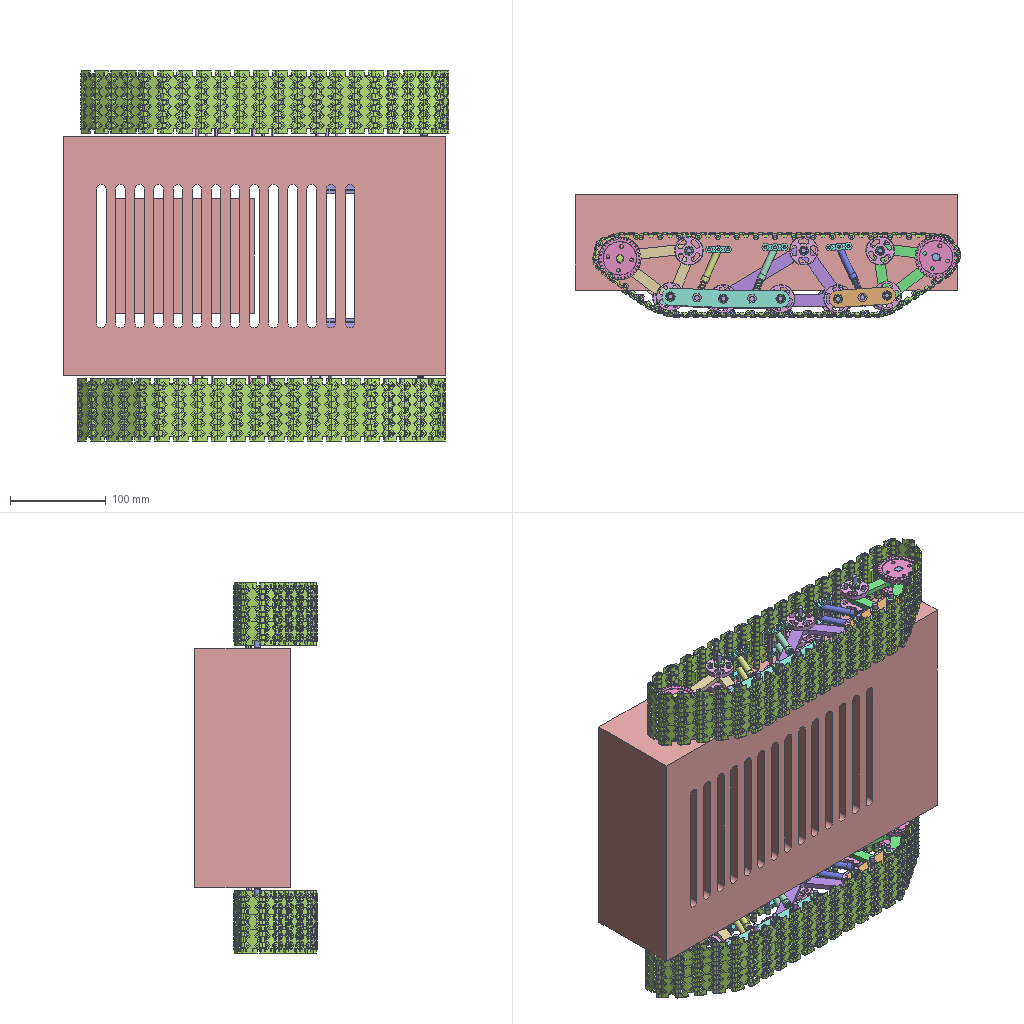Assembly | SolidWorks | 37 different items | 381 placed | box 403 x 128 x 388 mm
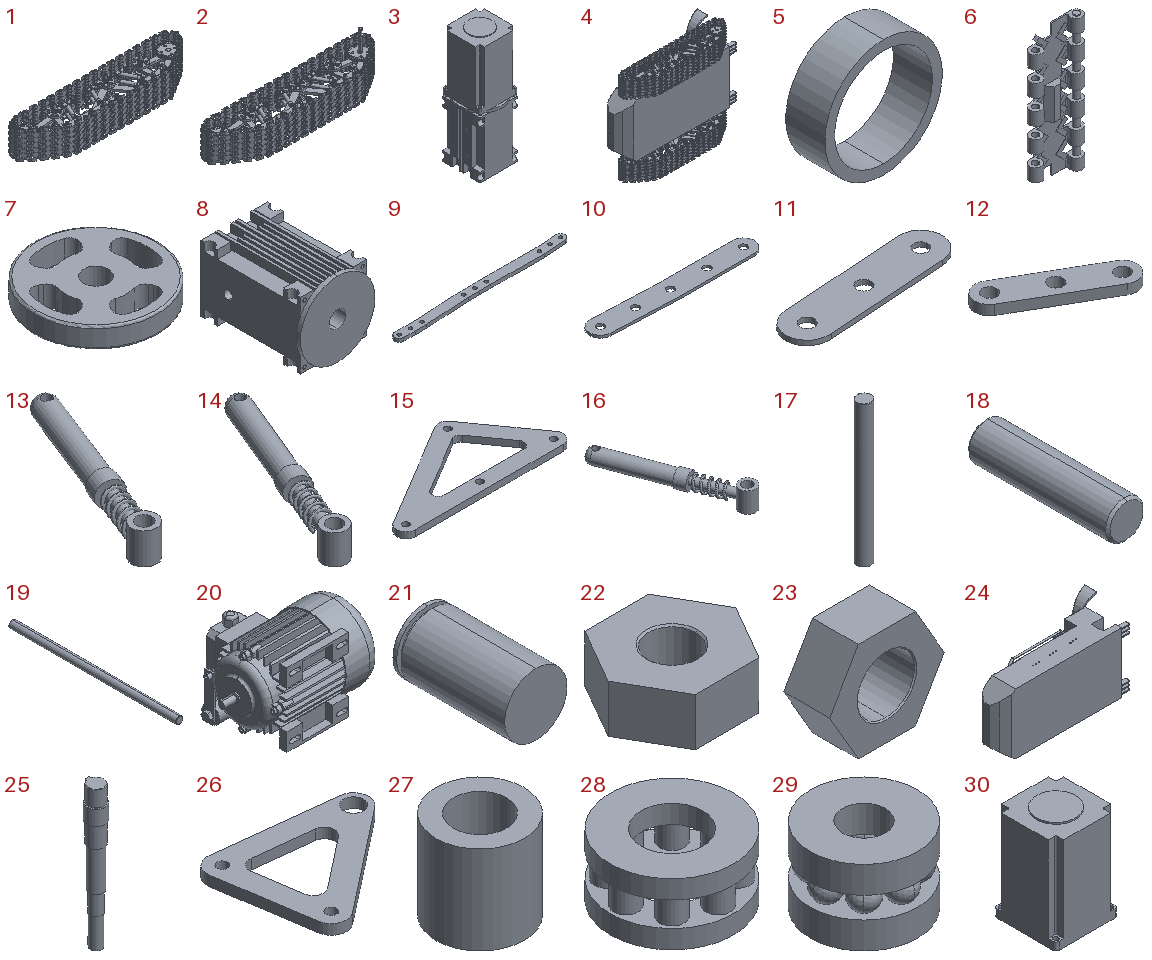Parts list (item | name | quantity | parent item | size | volume | features):
1 | (subassembly) | x1 | - | - | 270065 mm3 | features CompositeCurve 233, ReferencePattern 40, LocalChainPattern 1
2 | (subassembly) | x1 | - | - | 270065 mm3 | features CompositeCurve 245, ReferencePattern 40, LocalChainPattern 1
3 | (subassembly) | x1 | - | 45 x 45 x 123.5 mm | 175871 mm3 | -
4 | (subassembly) | x1 | - | - | 5126066 mm3 | features CompositeCurve 161, Cut 2
5 | - | x12 | in 1, 2 | 6 x 2 x 6 mm | 17.279 mm3 | features Extrusion 1
6 | - | x82 | in 1, 2 | 25.8 x 6.8 x 66 mm | 3099 mm3 | features ICE 7, Chamfer 1, Extrusion 1
7 | - | x32 | in 1, 2 | 30 x 30 x 5 mm | 2405 mm3 | features Extrusion 1, Fillet 1, ICE 1
8 | - | x1 | - | 45 x 62.5 x 45 mm | 83814 mm3 | features ICE 8, MirrorPattern 3, Extrusion 1
9 | - | x1 | - | 153.919 x 11.375 x 3 mm | 3465 mm3 | features Extrusion 1
10 | - | x4 | in 1, 2 | 133.234 x 20.271 x 2 mm | 4375 mm3 | features Extrusion 1
11 | - | x4 | in 1, 2 | 69.294 x 21.478 x 2 mm | 2186 mm3 | features Extrusion 1
12 | - | x12 | in 1, 2 | 23.321 x 16 x 2 mm | 254.137 mm3 | features Extrusion 1
13 | - | x4 | in 1, 2 | 28.061 x 59.393 x 10 mm | 2085 mm3 | features ICE 4, 3DProfileFeature 1, Extrusion 1, Fillet 1, Helix 1, Sweep 1
14 | - | x4 | in 1, 2 | 30.391 x 62.421 x 10 mm | 2131 mm3 | features ICE 4, 3DProfileFeature 2, Extrusion 1, Fillet 1, Helix 1, Sweep 1
15 | - | x2 | in 1, 2 | 135 x 65.308 x 5 mm | 17553 mm3 | features Extrusion 1
16 | - | x4 | in 1, 2 | 27.99 x 62.362 x 10 mm | 2119 mm3 | features ICE 4, 3DProfileFeature 2, Extrusion 1, Fillet 1, Helix 1, Sweep 1
17 | - | x22 | in 1, 2 | 5 x 5 x 50 mm | 981.593 mm3 | features Chamfer 1, Extrusion 1
18 | - | x2 | in 1, 2 | 8 x 30 x 8 mm | 1502 mm3 | features Chamfer 1, Extrusion 1
19 | - | x18 | - | 3 x 70 x 3 mm | 494.644 mm3 | features Extrusion 1, Fillet 1
20 | - | x1 | - | 53.612 x 38.693 x 34.5 mm | 25264 mm3 | features ICE 20, Fillet 3, CirPattern 2, Revolution 2, LPattern 1, Scale 1
21 | - | x1 | - | 150 x 290 x 150 mm | 4766313 mm3 | features ICE 3, Chamfer 1, Extrusion 1, Fillet 1
22 | - | x54 | - | 8 x 6.928 x 3 mm | 103.406 mm3 | features Chamfer 1, Extrusion 1
23 | - | x12 | in 1, 2 | 10 x 4 x 8.66 mm | 181.109 mm3 | features Chamfer 1, Extrusion 1
24 | - | x1 | - | 438.814 x 160 x 247.251 mm | 4513172 mm3 | features ICE 37, Fillet 7, Chamfer 2, 3DProfileFeature 1, BossThin 1, Extrusion 1, MirrorPattern 1, Shell 1, WeldMemberFeat 1, WeldmentFeature 1
25 | - | x2 | in 1, 2 | 9 x 9 x 71 mm | 2813 mm3 | features ICE 9, Chamfer 2, Fillet 2, Extrusion 1
26 | - | x2 | in 1, 2 | 73.414 x 61.829 x 5 mm | 9310 mm3 | features Extrusion 1
27 | - | x2 | - | 9.99 x 9.99 x 10 mm | 501.085 mm3 | features Extrusion 1
28 | - | x32 | in 1, 2 | 10 x 10 x 5 mm | 226.98 mm3 | features ICE 2, Extrusion 1
29 | - | x1 | - | 20 x 20 x 14 mm | 3133 mm3 | features CirPattern 1, Extrusion 1, ICE 1, Revolution 1
30 | - | x2 | - | 40 x 40 x 76 mm | 92058 mm3 | features ICE 4, Fillet 2, Extrusion 1
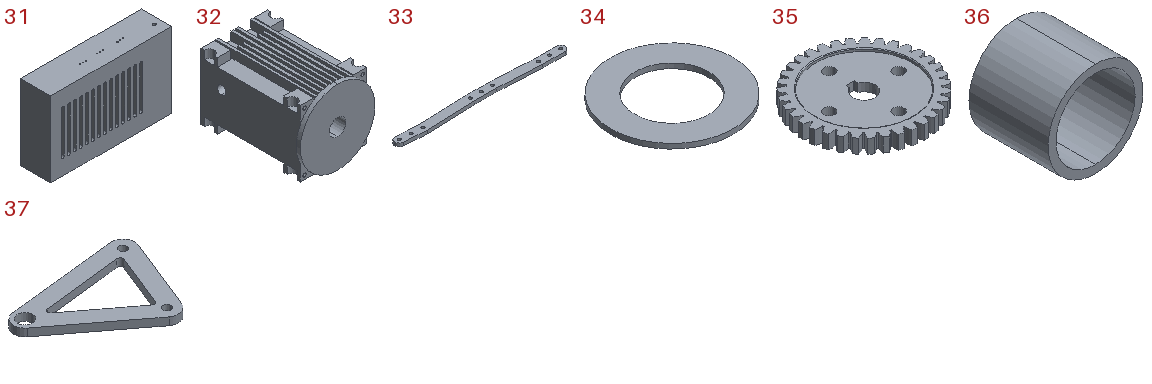31 | - | x1 | - | 400 x 100 x 250 mm | 2452161 mm3 | features ICE 7, Extrusion 1, Shell 1
32 | - | x1 | - | 45 x 62.5 x 45 mm | 83715 mm3 | features ICE 8, MirrorPattern 3, Extrusion 1
33 | - | x1 | - | 151.18 x 10.194 x 3 mm | 3447 mm3 | features Extrusion 1
34 | - | x18 | - | 5 x 5 x 0.2 mm | 2.513 mm3 | features Extrusion 1
35 | - | x8 | in 1, 2 | 44.212 x 44.202 x 5 mm | 4910 mm3 | features ICE 4, Fillet 2, Extrusion 1
36 | - | x32 | in 1, 2 | 6 x 5 x 6 mm | 43.197 mm3 | features Extrusion 1
37 | - | x2 | in 1, 2 | 87.181 x 63.036 x 5 mm | 10086 mm3 | features Extrusion 1
Mates (type | each side: item.copy, entity, surface, feature):
In the top assembly
Parallel | 31.1 edge | 10.1 edge
Concentric | 31.1 edge | 12.1 edge
Parallel | 31.1 edge | 15.1 edge
Concentric | 12.2 face cylinder Boss-Extrude1 | 19.1 edge
DistanceDim | 19.1 face plane Boss-Extrude1 | 12.2 face plane Boss-Extrude1
Concentric | 12.2 edge | 19.2 edge
DistanceDim | 19.2 face plane Boss-Extrude1 | 12.2 face plane Boss-Extrude1
Concentric | 12.2 edge | 19.3 edge
DistanceDim | 19.3 face plane Boss-Extrude1 | 12.2 face plane Boss-Extrude1
Concentric | 12.3 edge | 19.4 edge
DistanceDim | 19.4 face plane Boss-Extrude1 | 12.3 face plane Boss-Extrude1
Concentric | 12.3 edge | 19.5 edge
DistanceDim | 19.5 face plane Boss-Extrude1 | 12.3 face plane Boss-Extrude1
Concentric | 12.3 edge | 19.6 edge
DistanceDim | 19.6 face plane Boss-Extrude1 | 12.3 face plane Boss-Extrude1
Concentric | 12.4 edge | 19.7 edge
DistanceDim | 19.7 face plane Boss-Extrude1 | 12.4 face plane Boss-Extrude1
Concentric | 12.4 edge | 19.8 edge
DistanceDim | 19.8 face plane Boss-Extrude1 | 12.4 face plane Boss-Extrude1
Concentric | 12.4 edge | 19.9 edge
DistanceDim | 19.9 face plane Boss-Extrude1 | 12.4 face plane Boss-Extrude1
Concentric | 12.5 edge | 19.10 edge
DistanceDim | 19.10 face plane Boss-Extrude1 | 12.5 face plane Boss-Extrude1
DistanceDim | 19.9 face plane Boss-Extrude1 | 31.1 face plane
DistanceDim | 19.10 face plane Boss-Extrude1 | 31.1 face plane
Concentric | 12.5 edge | 19.11 edge
DistanceDim | 19.11 face plane Boss-Extrude1 | 12.5 face plane Boss-Extrude1
Concentric | 12.5 edge | 19.12 edge
DistanceDim | 19.12 face plane Boss-Extrude1 | 12.5 face plane Boss-Extrude1
Concentric | 12.6 edge | 19.13 edge
DistanceDim | 19.13 face plane Boss-Extrude1 | 12.6 face plane Boss-Extrude1
Concentric | 12.6 edge | 19.14 edge
DistanceDim | 19.14 face plane Boss-Extrude1 | 12.6 face plane Boss-Extrude1
Concentric | 12.6 edge | 19.15 edge
DistanceDim | 19.15 face plane Boss-Extrude1 | 12.6 face plane Boss-Extrude1
Concentric | 12.1 edge | 19.16 edge
DistanceDim | 19.16 face plane Boss-Extrude1 | 12.1 face plane Boss-Extrude1
Concentric | 12.1 edge | 19.17 edge
DistanceDim | 19.17 face plane Boss-Extrude1 | 12.1 face plane Boss-Extrude1
Concentric | 12.1 edge | 19.18 edge
DistanceDim | 19.18 face plane Boss-Extrude1 | 12.1 face plane Boss-Extrude1
Coincident | 12.2 face plane Boss-Extrude1 | 22.1 face plane Boss-Extrude1
Concentric | 12.2 edge | 22.1 edge
Coincident | 12.2 face plane Boss-Extrude1 | 22.2 face plane Boss-Extrude1
Concentric | 12.2 edge | 22.2 edge
Coincident | 12.2 face plane Boss-Extrude1 | 22.3 face plane Boss-Extrude1
Concentric | 12.2 edge | 22.3 edge
Coincident | 12.3 face plane Boss-Extrude1 | 22.4 face plane Boss-Extrude1
Concentric | 12.3 edge | 22.4 edge
Coincident | 12.3 face plane Boss-Extrude1 | 22.5 face plane Boss-Extrude1
Concentric | 12.3 edge | 22.5 edge
Coincident | 12.3 face plane Boss-Extrude1 | 22.6 face plane Boss-Extrude1
Concentric | 19.6 edge | 22.6 edge
Coincident | 12.4 face plane Boss-Extrude1 | 22.7 face plane Boss-Extrude1
Concentric | 12.4 edge | 22.7 edge
Coincident | 12.4 face plane Boss-Extrude1 | 22.8 face plane Boss-Extrude1
Concentric | 19.8 face cylinder Boss-Extrude1 | 22.8 edge
Coincident | 12.4 face plane Boss-Extrude1 | 22.9 face plane Boss-Extrude1
Concentric | 12.4 edge | 22.9 edge
Coincident | 12.7 face plane Boss-Extrude1 | 22.10 face plane Boss-Extrude1
Concentric | 19.1 face cylinder Boss-Extrude1 | 22.10 edge
Coincident | 12.7 face plane Boss-Extrude1 | 22.11 face plane Boss-Extrude1
Concentric | 19.2 face cylinder Boss-Extrude1 | 22.11 edge
Coincident | 12.7 face plane Boss-Extrude1 | 22.12 face plane Boss-Extrude1
Concentric | 19.3 face cylinder Boss-Extrude1 | 22.12 face cone Chamfer1
Coincident | 12.8 face plane Boss-Extrude1 | 22.13 face plane Boss-Extrude1
Concentric | 19.4 face cylinder Boss-Extrude1 | 22.13 edge
Coincident | 12.8 face plane Boss-Extrude1 | 22.14 face plane Boss-Extrude1
Concentric | 19.5 face cylinder Boss-Extrude1 | 22.14 edge
Coincident | 12.8 face plane Boss-Extrude1 | 22.15 face plane Boss-Extrude1
Concentric | 19.6 face cylinder Boss-Extrude1 | 22.15 edge
Coincident | 12.9 face plane Boss-Extrude1 | 22.16 face plane Boss-Extrude1
Concentric | 19.7 face cylinder Boss-Extrude1 | 22.16 edge
Coincident | 12.9 face plane Boss-Extrude1 | 22.17 face plane Boss-Extrude1
Concentric | 19.8 face cylinder Boss-Extrude1 | 22.17 edge
Coincident | 12.9 face plane Boss-Extrude1 | 22.18 face plane Boss-Extrude1
Concentric | 19.9 face cylinder Boss-Extrude1 | 22.18 edge
Coincident | 12.5 face plane Boss-Extrude1 | 22.19 face plane Boss-Extrude1
Concentric | 19.10 face cylinder Boss-Extrude1 | 22.19 edge
Coincident | 12.5 face plane Boss-Extrude1 | 22.20 face plane Boss-Extrude1
Concentric | 19.11 face cylinder Boss-Extrude1 | 22.20 edge
Coincident | 12.5 face plane Boss-Extrude1 | 22.21 face plane Boss-Extrude1
Concentric | 19.12 face cylinder Boss-Extrude1 | 22.21 edge
Coincident | 12.6 face plane Boss-Extrude1 | 22.22 face plane Boss-Extrude1
Concentric | 19.13 face cylinder Boss-Extrude1 | 22.22 edge
Coincident | 12.6 face plane Boss-Extrude1 | 22.23 face plane Boss-Extrude1
Concentric | 19.14 face cylinder Boss-Extrude1 | 22.23 edge
Coincident | 12.6 face plane Boss-Extrude1 | 22.24 face plane Boss-Extrude1
Concentric | 19.15 face cylinder Boss-Extrude1 | 22.24 edge
Coincident | 12.1 face plane Boss-Extrude1 | 22.25 face plane Boss-Extrude1
Concentric | 19.16 face cylinder Boss-Extrude1 | 22.25 edge
Coincident | 12.1 face plane Boss-Extrude1 | 22.26 face plane Boss-Extrude1
Concentric | 19.17 face cylinder Boss-Extrude1 | 22.26 edge
Coincident | 12.1 face plane Boss-Extrude1 | 22.27 face plane Boss-Extrude1
Concentric | 19.18 face cylinder Boss-Extrude1 | 22.27 face cone Chamfer1
Coincident | 12.10 face plane Boss-Extrude1 | 22.28 face plane Boss-Extrude1
Concentric | 19.10 face cylinder Boss-Extrude1 | 22.28 edge
Coincident | 12.10 face plane Boss-Extrude1 | 22.29 face plane Boss-Extrude1
Concentric | 19.11 face cylinder Boss-Extrude1 | 22.29 edge
Coincident | 12.10 face plane Boss-Extrude1 | 22.30 face plane Boss-Extrude1
Concentric | 19.12 face cylinder Boss-Extrude1 | 22.30 edge
Coincident | 12.11 face plane Boss-Extrude1 | 22.31 face plane Boss-Extrude1
Concentric | 19.13 face cylinder Boss-Extrude1 | 22.31 edge
Coincident | 12.11 face plane Boss-Extrude1 | 22.32 face plane Boss-Extrude1
Concentric | 19.14 face cylinder Boss-Extrude1 | 22.32 edge
Coincident | 12.11 face plane Boss-Extrude1 | 22.33 face plane Boss-Extrude1
Concentric | 19.15 face cylinder Boss-Extrude1 | 22.33 edge
Coincident | 12.12 face plane Boss-Extrude1 | 22.34 face plane Boss-Extrude1
Concentric | 19.16 face cylinder Boss-Extrude1 | 22.34 edge
Coincident | 12.12 face plane Boss-Extrude1 | 22.35 face plane Boss-Extrude1
Concentric | 19.17 face cylinder Boss-Extrude1 | 22.35 edge
Coincident | 12.12 face plane Boss-Extrude1 | 22.36 face plane Boss-Extrude1
Concentric | 19.18 face cylinder Boss-Extrude1 | 22.36 edge
Concentric | 31.1 face cylinder Cut-Extrude1 | 19.1 face cylinder Boss-Extrude1
Concentric | 31.1 edge | 19.2 face cylinder Boss-Extrude1
Concentric | 31.1 edge | 19.3 face cylinder Boss-Extrude1
Concentric | 19.10 face cylinder Boss-Extrude1 | 34.1 edge
Coincident | 31.1 face plane | 34.1 face plane Boss-Extrude1
Coincident | 31.1 face plane | 34.2 face plane Boss-Extrude1
Concentric | 19.11 face cylinder Boss-Extrude1 | 34.2 edge
Coincident | 31.1 face plane | 34.3 face plane Boss-Extrude1
Concentric | 19.12 face cylinder Boss-Extrude1 | 34.3 face cylinder Boss-Extrude1
Coincident | 31.1 face plane | 34.4 face plane Boss-Extrude1
Concentric | 19.13 face cylinder Boss-Extrude1 | 34.4 edge
Coincident | 31.1 face plane | 34.5 face plane Boss-Extrude1
Concentric | 19.14 face cylinder Boss-Extrude1 | 34.5 edge
Coincident | 31.1 face plane | 34.6 face plane Boss-Extrude1
Concentric | 19.15 face cylinder Boss-Extrude1 | 34.6 edge
Coincident | 31.1 face plane | 34.7 face plane Boss-Extrude1
Concentric | 19.16 face cylinder Boss-Extrude1 | 34.7 edge
Coincident | 31.1 face plane | 34.8 face plane Boss-Extrude1
Concentric | 19.17 face cylinder Boss-Extrude1 | 34.8 edge
Coincident | 31.1 face plane | 34.9 face plane Boss-Extrude1
Concentric | 19.18 face cylinder Boss-Extrude1 | 34.9 edge
Coincident | 31.1 face plane | 34.10 face plane Boss-Extrude1
Concentric | 19.9 face cylinder Boss-Extrude1 | 34.10 edge
Coincident | 31.1 face plane | 34.11 face plane Boss-Extrude1
Concentric | 19.8 face cylinder Boss-Extrude1 | 34.11 edge
Coincident | 31.1 face plane | 34.12 face plane Boss-Extrude1
Concentric | 19.7 face cylinder Boss-Extrude1 | 34.12 edge
Coincident | 31.1 face plane | 34.13 face plane Boss-Extrude1
Concentric | 19.6 face cylinder Boss-Extrude1 | 34.13 edge
Coincident | 31.1 face plane | 34.14 edge
Concentric | 19.5 face cylinder Boss-Extrude1 | 34.14 edge
Coincident | 31.1 face plane | 34.15 face plane Boss-Extrude1
Concentric | 19.4 face cylinder Boss-Extrude1 | 34.15 edge
Coincident | 31.1 face plane | 34.16 face plane Boss-Extrude1
Concentric | 19.3 face cylinder Boss-Extrude1 | 34.16 edge
Coincident | 31.1 face plane | 34.17 face plane Boss-Extrude1
Concentric | 19.2 face cylinder Boss-Extrude1 | 34.17 edge
Coincident | 31.1 face plane | 34.18 face plane Boss-Extrude1
Concentric | 19.1 face cylinder Boss-Extrude1 | 34.18 edge
Coincident | 34.1 face plane Boss-Extrude1 | 22.37 face plane Boss-Extrude1
Concentric | 19.10 face cylinder Boss-Extrude1 | 22.37 edge
Coincident | 34.2 face plane Boss-Extrude1 | 22.38 face plane Boss-Extrude1
Concentric | 19.11 face cylinder Boss-Extrude1 | 22.38 edge
Coincident | 34.3 face plane Boss-Extrude1 | 22.39 face plane Boss-Extrude1
Concentric | 19.12 face cylinder Boss-Extrude1 | 22.39 edge
Coincident | 34.4 face plane Boss-Extrude1 | 22.40 face plane Boss-Extrude1
Concentric | 19.13 face cylinder Boss-Extrude1 | 22.40 edge
Coincident | 34.5 face plane Boss-Extrude1 | 22.41 face plane Boss-Extrude1
Concentric | 19.14 face cylinder Boss-Extrude1 | 22.41 edge
Coincident | 34.6 face plane Boss-Extrude1 | 22.42 face plane Boss-Extrude1
Concentric | 19.15 face cylinder Boss-Extrude1 | 22.42 edge
Coincident | 34.7 face plane Boss-Extrude1 | 22.43 face plane Boss-Extrude1
Concentric | 19.16 face cylinder Boss-Extrude1 | 22.43 edge
Coincident | 34.8 face plane Boss-Extrude1 | 22.44 face plane Boss-Extrude1
Concentric | 19.17 face cylinder Boss-Extrude1 | 22.44 edge
Coincident | 34.9 face plane Boss-Extrude1 | 22.45 face plane Boss-Extrude1
Concentric | 19.18 face cylinder Boss-Extrude1 | 22.45 edge
Coincident | 34.10 face plane Boss-Extrude1 | 22.46 face plane Boss-Extrude1
Concentric | 19.9 face cylinder Boss-Extrude1 | 22.46 edge
Coincident | 34.11 face plane Boss-Extrude1 | 22.47 face plane Boss-Extrude1
Concentric | 19.8 face cylinder Boss-Extrude1 | 22.47 edge
Coincident | 34.12 face plane Boss-Extrude1 | 22.48 face plane Boss-Extrude1
Concentric | 19.7 face cylinder Boss-Extrude1 | 22.48 edge
Coincident | 34.13 face plane Boss-Extrude1 | 22.49 face plane Boss-Extrude1
Concentric | 19.6 face cylinder Boss-Extrude1 | 22.49 edge
Coincident | 34.14 face plane Boss-Extrude1 | 22.50 face plane Boss-Extrude1
Concentric | 19.5 face cylinder Boss-Extrude1 | 22.50 edge
Coincident | 34.15 face plane Boss-Extrude1 | 22.51 face plane Boss-Extrude1
Concentric | 19.4 face cylinder Boss-Extrude1 | 22.51 edge
Coincident | 34.16 face plane Boss-Extrude1 | 22.52 face plane Boss-Extrude1
Concentric | 19.3 face cylinder Boss-Extrude1 | 22.52 edge
Coincident | 34.17 face plane Boss-Extrude1 | 22.53 face plane Boss-Extrude1
Concentric | 19.2 face cylinder Boss-Extrude1 | 22.53 edge
Coincident | 34.18 face plane Boss-Extrude1 | 22.54 face plane Boss-Extrude1
Concentric | 19.1 face cylinder Boss-Extrude1 | 22.54 edge
Parallel | 31.1 edge | 30.1 edge
Coincident | 31.1 face plane | 30.1 face plane Boss-Extrude1
Concentric | 32.1 edge | 30.2 edge
Coincident | 32.1 face plane Boss-Extrude3 | 30.2 face plane Boss-Extrude1
Coincident | 32.1 edge | 30.2 edge
Coincident | 31.1 face plane | 30.2 face plane Boss-Extrude1
Coincident | 31.1 face plane | 32.1 face plane Boss-Extrude1
DistanceDim | 32.1 face plane Boss-Extrude1 | 31.1 face plane
Concentric | 30.1 edge | 8.1 edge
Coincident | 30.1 face plane Boss-Extrude1 | 8.1 face plane Boss-Extrude3
Coincident | 30.1 edge | 8.1 edge
Coincident | 31.1 face plane | 8.1 face plane Boss-Extrude1
DistanceDim | 8.1 face plane Boss-Extrude1 | 31.1 face plane
Concentric | 31.1 edge | 27.1 edge
Coincident | 31.1 face plane | 27.1 face plane Boss-Extrude1
Concentric | 31.1 edge | 27.2 edge
Coincident | 31.1 face plane | 27.2 face plane Boss-Extrude1
In subassembly 2
Parallel | 6.1 face plane Boss-Extrude3 | 7.1 face plane Boss-Extrude1
Coincident | 6.1 face plane Boss-Extrude3 | 7.1 face plane Boss-Extrude1
Tangent | 6.1 face cylinder Boss-Extrude1 | 7.1 face cylinder Boss-Extrude1
Parallel | 6.1 face plane Boss-Extrude3 | 7.2 face plane Boss-Extrude1
Coincident | 6.1 face plane Boss-Extrude3 | 7.2 face plane Boss-Extrude1
Tangent | 6.2 face cylinder Boss-Extrude1 | 7.2 face cylinder Boss-Extrude1
Tangent | 6.1 face cylinder Boss-Extrude1 | 7.2 face cylinder Boss-Extrude1
Coincident | 6.3 face plane Boss-Extrude3 | 7.3 face plane Boss-Extrude1
Tangent | 6.3 face cylinder Boss-Extrude1 | 7.3 face cylinder Boss-Extrude1
Tangent | 6.4 face cylinder Boss-Extrude1 | 7.3 face cylinder Boss-Extrude1
Coincident | 6.3 face plane Boss-Extrude3 | 7.4 face plane Boss-Extrude1
Tangent | 6.3 face cylinder Boss-Extrude1 | 7.4 face cylinder Boss-Extrude1
Tangent | 6.5 face cylinder Boss-Extrude1 | 7.4 face cylinder Boss-Extrude1
Concentric | 7.4 edge | 7.3 edge
Tangent | 6.6 face cylinder Boss-Extrude1 | 7.5 face cylinder Boss-Extrude1
Tangent | 6.7 face cylinder Boss-Extrude1 | 7.5 face cylinder Boss-Extrude1 | 2 times
Coincident | 6.6 face plane Boss-Extrude3 | 7.6 face plane Boss-Extrude1
Tangent | 6.7 face cylinder Boss-Extrude1 | 7.6 face cylinder Boss-Extrude1
Tangent | 6.8 face cylinder Boss-Extrude1 | 7.6 face cylinder Boss-Extrude1
Coincident | 6.6 face plane Boss-Extrude3 | 7.5 face plane Boss-Extrude1
Tangent | 6.8 face cylinder Boss-Extrude1 | 7.5 face cylinder Boss-Extrude1
Concentric | 7.6 edge | 7.5 edge
Coincident | 6.9 face plane Boss-Extrude3 | 7.7 face plane Boss-Extrude1
Tangent | 6.9 face cylinder Boss-Extrude1 | 7.7 face cylinder Boss-Extrude1 | 2 times
Coincident | 6.9 face plane Boss-Extrude3 | 7.8 face plane Boss-Extrude1
Tangent | 6.9 face cylinder Boss-Extrude1 | 7.8 face cylinder Boss-Extrude1 | 2 times
Coincident | 6.10 face plane Boss-Extrude3 | 7.9 face plane Boss-Extrude1
Coincident | 6.11 edge | 7.10 face plane Boss-Extrude1
Tangent | 6.11 face cylinder Boss-Extrude1 | 7.10 face cylinder Boss-Extrude1
Parallel | 6.12 face plane Boss-Extrude3 | 7.10 face plane Boss-Extrude1
Tangent | 6.13 face cylinder Boss-Extrude1 | 7.10 face cylinder Boss-Extrude1
Coincident | 6.11 face plane Boss-Extrude3 | 7.11 face plane Boss-Extrude1
Tangent | 6.11 face cylinder Boss-Extrude1 | 7.11 face cylinder Boss-Extrude1
Tangent | 6.13 face cylinder Boss-Extrude1 | 7.11 face cylinder Boss-Extrude1
Tangent | 6.2 face cylinder Boss-Extrude1 | 7.1 face cylinder Boss-Extrude1
Coincident | 6.10 face plane Boss-Extrude3 | 7.12 face plane Boss-Extrude1
Tangent | 6.10 face cylinder Boss-Extrude1 | 7.12 face cylinder Boss-Extrude1 | 2 times
Coincident | 6.14 edge | 7.13 face plane Boss-Extrude1
Parallel | 6.15 face plane Boss-Extrude3 | 7.13 face plane Boss-Extrude1
Tangent | 6.16 face cylinder Boss-Extrude1 | 7.13 face cylinder Boss-Extrude1
Tangent | 6.14 face cylinder Boss-Extrude1 | 7.13 face cylinder Boss-Extrude1
Coincident | 6.14 face plane Boss-Extrude3 | 7.14 face plane Boss-Extrude1
Tangent | 6.14 face cylinder Boss-Extrude1 | 7.14 face cylinder Boss-Extrude1
Tangent | 6.16 face cylinder Boss-Extrude1 | 7.14 face cylinder Boss-Extrude1
Concentric | 7.1 edge | 7.2 edge
Tangent | 6.17 face cylinder Boss-Extrude1 | 7.9 face cylinder Boss-Extrude1
Tangent | 6.10 face cylinder Boss-Extrude1 | 7.9 face cylinder Boss-Extrude1
Concentric | 7.13 edge | 7.14 edge
Coincident | 7.1 face plane Boss-Extrude1 | 10.2 face plane Boss-Extrude1
Concentric | 7.1 edge | 10.2 edge
Concentric | 7.9 edge | 10.2 edge
Coincident | 7.2 face plane Boss-Extrude1 | 10.3 face plane Boss-Extrude1
Concentric | 7.2 edge | 10.3 edge
Coincident | 7.11 face plane Boss-Extrude1 | 11.1 face plane Boss-Extrude1
Concentric | 7.4 edge | 11.1 edge
Concentric | 7.3 edge | 11.2 edge
Coincident | 7.3 face plane Boss-Extrude1 | 11.2 face plane Boss-Extrude1
Concentric | 10.2 edge | 17.1 edge
DistanceDim | 17.1 face plane Boss-Extrude1 | 10.2 face plane Boss-Extrude1
Concentric | 10.2 edge | 17.2 edge
DistanceDim | 17.2 face plane Boss-Extrude1 | 10.2 face plane Boss-Extrude1
Concentric | 10.2 edge | 17.3 face cone Chamfer1
DistanceDim | 17.3 face plane Boss-Extrude1 | 10.2 face plane Boss-Extrude1
Concentric | 10.2 edge | 17.4 edge
DistanceDim | 17.4 face plane Boss-Extrude1 | 10.2 face plane Boss-Extrude1
Concentric | 10.2 edge | 17.5 edge
DistanceDim | 17.5 face plane Boss-Extrude1 | 10.2 face plane Boss-Extrude1
Concentric | 11.2 edge | 17.6 edge
DistanceDim | 17.6 face plane Boss-Extrude1 | 11.2 face plane Boss-Extrude1
Concentric | 11.2 edge | 17.7 edge
DistanceDim | 17.7 face plane Boss-Extrude1 | 11.2 face plane Boss-Extrude1
Concentric | 17.1 edge | 28.1 edge
Coincident | 10.2 face plane Boss-Extrude1 | 28.1 face plane Boss-Extrude2
Concentric | 17.3 edge | 28.2 edge
Coincident | 10.2 face plane Boss-Extrude1 | 28.2 face plane Boss-Extrude2
Concentric | 17.5 edge | 28.3 edge
Coincident | 10.2 face plane Boss-Extrude1 | 28.3 face plane Boss-Extrude2
Concentric | 17.6 edge | 28.4 edge
Coincident | 11.2 face plane Boss-Extrude1 | 28.4 face plane Boss-Extrude2
Concentric | 17.7 edge | 28.5 edge
Coincident | 11.2 face plane Boss-Extrude1 | 28.5 face plane Boss-Extrude2
Concentric | 17.7 edge | 28.6 edge
Coincident | 11.1 face plane Boss-Extrude1 | 28.6 face plane Boss-Extrude1
Concentric | 17.5 edge | 28.7 edge
Coincident | 10.3 face plane Boss-Extrude1 | 28.7 face plane Boss-Extrude1
Concentric | 17.6 edge | 28.8 edge
Coincident | 11.1 face plane Boss-Extrude1 | 28.8 face plane Boss-Extrude1
Concentric | 17.3 edge | 28.9 edge
Coincident | 10.3 face plane Boss-Extrude1 | 28.9 face plane Boss-Extrude1
Concentric | 17.1 edge | 28.10 edge
Coincident | 10.3 face plane Boss-Extrude1 | 28.10 face plane Boss-Extrude1
Concentric | 17.1 edge | 36.1 edge
Coincident | 7.1 face plane Boss-Extrude1 | 36.1 face plane Boss-Extrude1
Concentric | 17.1 edge | 36.2 edge
Coincident | 7.2 face plane Boss-Extrude1 | 36.2 face plane Boss-Extrude1
Concentric | 17.3 edge | 36.3 edge
Coincident | 7.14 face plane Boss-Extrude1 | 36.3 face plane Boss-Extrude1
Concentric | 17.5 edge | 36.4 edge
Coincident | 7.12 face plane Boss-Extrude1 | 36.4 face plane Boss-Extrude1
Concentric | 17.6 edge | 36.5 edge
Coincident | 7.11 face plane Boss-Extrude1 | 36.5 edge
Concentric | 17.7 edge | 36.6 edge
Coincident | 7.4 face plane Boss-Extrude1 | 36.6 face plane Boss-Extrude1
Concentric | 17.7 edge | 36.7 edge
Coincident | 7.3 face plane Boss-Extrude1 | 36.7 face plane Boss-Extrude1
Concentric | 17.6 edge | 36.8 edge
Coincident | 7.10 face plane Boss-Extrude1 | 36.8 face plane Boss-Extrude1
Concentric | 17.5 edge | 36.9 edge
Coincident | 7.9 face plane Boss-Extrude1 | 36.9 face plane Boss-Extrude1
Concentric | 28.2 edge | 36.10 edge
Coincident | 7.13 face plane Boss-Extrude1 | 36.10 face plane Boss-Extrude1
Concentric | 17.2 edge | 5.1 edge
Coincident | 10.2 face plane Boss-Extrude1 | 5.1 face plane Boss-Extrude1
Concentric | 17.4 edge | 5.2 edge
Coincident | 10.2 face plane Boss-Extrude1 | 5.2 face plane Boss-Extrude1
Concentric | 17.4 edge | 5.3 edge
Coincident | 10.3 face plane Boss-Extrude1 | 5.3 face plane Boss-Extrude1
Concentric | 17.2 edge | 5.4 edge
Coincident | 10.3 face plane Boss-Extrude1 | 5.4 face plane Boss-Extrude1
Concentric | 10.2 edge | 13.1 edge
Coincident | 10.2 face plane Boss-Extrude1 | 13.1 face plane Boss-Extrude1
Concentric | 5.4 edge | 13.2 edge
Coincident | 10.3 face plane Boss-Extrude1 | 13.2 face plane Boss-Extrude1
Concentric | 17.4 edge | 14.1 edge
Coincident | 10.2 face plane Boss-Extrude1 | 14.1 face plane Boss-Extrude1
Concentric | 17.4 edge | 14.2 edge
Coincident | 10.3 face plane Boss-Extrude1 | 14.2 face plane Boss-Extrude1
Parallel | 14.1 face cylinder Boss-Extrude2 | 14.2 face cylinder Boss-Extrude2
Coincident | 6.18 face plane Boss-Extrude3 | 7.15 face plane Boss-Extrude1
Tangent | 6.19 face cylinder Boss-Extrude1 | 7.15 face cylinder Boss-Extrude1 | 2 times
Coincident | 6.20 face plane Boss-Extrude3 | 7.16 face plane Boss-Extrude1
Tangent | 6.21 face cylinder Boss-Extrude1 | 7.16 face cylinder Boss-Extrude1
Tangent | 6.20 face cylinder Boss-Extrude1 | 7.16 face cylinder Boss-Extrude1
Concentric | 11.2 edge | 17.8 edge
DistanceDim | 17.8 face plane Boss-Extrude1 | 11.2 face plane Boss-Extrude1
Concentric | 17.8 edge | 5.5 edge
Coincident | 11.2 face plane Boss-Extrude1 | 5.5 face plane Boss-Extrude1
Concentric | 17.8 edge | 5.6 edge
Coincident | 11.1 face plane Boss-Extrude1 | 5.6 face plane Boss-Extrude1
Concentric | 17.8 edge | 16.1 edge
Coincident | 11.2 face plane Boss-Extrude1 | 16.1 face plane Boss-Extrude1
Concentric | 17.8 edge | 16.2 edge
Coincident | 11.1 face plane Boss-Extrude1 | 16.2 face plane Boss-Extrude1
Concentric | 7.6 edge | 17.9 edge
DistanceDim | 17.9 face plane Boss-Extrude1 | 7.5 face plane Boss-Extrude1
Concentric | 7.16 edge | 17.10 edge
DistanceDim | 17.10 face plane Boss-Extrude1 | 7.16 face plane Boss-Extrude1
Concentric | 7.8 edge | 17.11 edge
DistanceDim | 17.11 face plane Boss-Extrude1 | 7.8 face plane Boss-Extrude1
Concentric | 17.11 edge | 36.11 edge
Coincident | 7.8 face plane Boss-Extrude1 | 36.11 face plane Boss-Extrude1
Concentric | 17.11 face cone Chamfer1 | 36.12 edge
Coincident | 7.7 face plane Boss-Extrude1 | 36.12 face plane Boss-Extrude1
Concentric | 7.15 edge | 36.13 edge
Coincident | 7.15 face plane Boss-Extrude1 | 36.13 face plane Boss-Extrude1
Concentric | 7.16 edge | 36.14 edge
Coincident | 7.16 face plane Boss-Extrude1 | 36.14 face plane Boss-Extrude1
Concentric | 7.5 edge | 36.15 edge
Coincident | 7.5 face plane Boss-Extrude1 | 36.15 face plane Boss-Extrude1
Concentric | 17.9 face cone Chamfer1 | 36.16 edge
Coincident | 7.6 face plane Boss-Extrude1 | 36.16 face plane Boss-Extrude1
Concentric | 17.10 edge | 28.11 edge
Coincident | 7.15 face plane Boss-Extrude1 | 28.11 face plane Boss-Extrude2
Concentric | 17.10 edge | 28.12 edge
Coincident | 7.16 face plane Boss-Extrude1 | 28.12 face plane Boss-Extrude1
Concentric | 17.11 edge | 28.13 edge
Coincident | 7.8 face plane Boss-Extrude1 | 28.13 face plane Boss-Extrude1
Concentric | 17.11 edge | 28.14 edge
Coincident | 7.7 face plane Boss-Extrude1 | 28.14 face plane Boss-Extrude2
Concentric | 17.9 edge | 28.15 edge
Coincident | 7.6 face plane Boss-Extrude1 | 28.15 face plane Boss-Extrude2
Concentric | 17.9 edge | 28.16 edge
Coincident | 7.5 face plane Boss-Extrude1 | 28.16 face plane Boss-Extrude1
Concentric | 13.2 face cylinder Cut-Extrude1 | 13.1 face cylinder Cut-Extrude1
Concentric | 7.10 edge | 17.6 edge
Concentric | 16.1 face cylinder Cut-Extrude1 | 16.2 face cylinder Cut-Extrude1
Parallel | 13.1 face cylinder Boss-Extrude2 | 14.1 face cylinder Boss-Extrude2
Concentric | 13.1 face cylinder Cut-Extrude1 | 12.13 edge
Tangent | 13.2 face cylinder Boss-Extrude2 | 12.13 face plane Boss-Extrude1
Concentric | 13.1 face cylinder Cut-Extrude1 | 12.14 face cylinder Boss-Extrude1
Tangent | 13.1 face cylinder Boss-Extrude2 | 12.14 face plane Boss-Extrude1
Concentric | 14.1 face cylinder Cut-Extrude1 | 12.15 face cylinder Boss-Extrude1
Tangent | 14.2 face cylinder Boss-Extrude2 | 12.15 face plane Boss-Extrude1
Concentric | 14.1 face cylinder Cut-Extrude1 | 12.16 face cylinder Boss-Extrude1
Tangent | 14.1 face cylinder Boss-Extrude2 | 12.16 face plane Boss-Extrude1
Concentric | 16.1 face cylinder Cut-Extrude1 | 12.17 face cylinder Boss-Extrude1
Tangent | 16.2 face cylinder Boss-Extrude2 | 12.17 face plane Boss-Extrude1
Concentric | 16.1 face cylinder Cut-Extrude1 | 12.18 face cylinder Boss-Extrude1
Tangent | 16.1 face cylinder Boss-Extrude2 | 12.18 face plane Boss-Extrude1
Concentric | 17.9 edge | 37.1 edge
Concentric | 17.1 edge | 37.1 edge
Concentric | 17.10 edge | 15.2 edge
Concentric | 17.3 edge | 15.2 edge
Concentric | 15.2 edge | 17.5 edge
Concentric | 17.6 edge | 15.2 edge
DistanceDim | 15.2 face plane Boss-Extrude1 | 7.15 face plane Boss-Extrude1
Concentric | 17.7 edge | 26.1 edge
Concentric | 17.11 edge | 26.1 edge
DistanceDim | 26.1 face plane Boss-Extrude1 | 7.8 face plane Boss-Extrude1
Concentric | 12.17 edge | 12.18 edge
Concentric | 12.13 edge | 12.14 edge
Concentric | 12.15 edge | 12.16 edge
Parallel | 10.2 edge | 12.14 edge
Parallel | 10.2 edge | 12.16 edge
Parallel | 11.2 edge | 12.18 edge
Concentric | 37.1 edge | 35.1 edge
Concentric | 26.1 edge | 35.2 edge | 2 times
Concentric | 35.1 edge | 35.3 edge | 3 times
Concentric | 17.2 face cylinder Boss-Extrude1 | 23.1 edge
Coincident | 10.3 face plane Boss-Extrude1 | 23.1 face plane Boss-Extrude1
Concentric | 17.2 face cylinder Boss-Extrude1 | 23.2 edge
Coincident | 10.2 face plane Boss-Extrude1 | 23.2 face plane Boss-Extrude1
Concentric | 17.4 face cylinder Boss-Extrude1 | 23.3 edge
Coincident | 10.2 face plane Boss-Extrude1 | 23.3 face plane Boss-Extrude1
Concentric | 17.4 face cylinder Boss-Extrude1 | 23.4 edge
Coincident | 10.3 face plane Boss-Extrude1 | 23.4 face plane Boss-Extrude1
Concentric | 17.8 face cylinder Boss-Extrude1 | 23.5 edge
Coincident | 11.1 face plane Boss-Extrude1 | 23.5 face plane Boss-Extrude1
Concentric | 17.8 face cylinder Boss-Extrude1 | 23.6 edge
Coincident | 11.2 face plane Boss-Extrude1 | 23.6 face plane Boss-Extrude1
Concentric | 37.1 edge | 35.3 edge
DistanceDim | 35.1 face plane Boss-Extrude1 | 37.1 face plane Boss-Extrude1
DistanceDim | 37.1 face plane Boss-Extrude1 | 35.3 face plane Boss-Extrude1
DistanceDim | 37.1 face plane Boss-Extrude1 | 7.2 face plane Boss-Extrude1
Concentric | 26.1 edge | 35.4 edge
DistanceDim | 35.2 face plane Boss-Extrude1 | 26.1 face plane Boss-Extrude1
DistanceDim | 26.1 face plane Boss-Extrude1 | 35.4 face plane Boss-Extrude1
Coincident | 35.2 face plane Cut-Extrude4 | 25.1 face plane Boss-Extrude1
Concentric | 35.3 edge | 18.1 edge
DistanceDim | 18.1 face plane Boss-Extrude1 | 35.3 face plane Cut-Extrude4
Concentric | 35.2 edge | 35.4 edge
Concentric | 26.1 edge | 25.1 edge
Parallel | 35.2 edge | 25.1 edge
In subassembly 1
Parallel | 6.1 face plane Boss-Extrude3 | 7.1 face plane Boss-Extrude1
Coincident | 6.1 face plane Boss-Extrude3 | 7.1 face plane Boss-Extrude1
Tangent | 6.1 face cylinder Boss-Extrude1 | 7.1 face cylinder Boss-Extrude1
Parallel | 6.1 face plane Boss-Extrude3 | 7.2 face plane Boss-Extrude1
Coincident | 6.1 face plane Boss-Extrude3 | 7.2 face plane Boss-Extrude1
Tangent | 6.2 face cylinder Boss-Extrude1 | 7.2 face cylinder Boss-Extrude1
Tangent | 6.1 face cylinder Boss-Extrude1 | 7.2 face cylinder Boss-Extrude1
Coincident | 6.3 face plane Boss-Extrude3 | 7.3 face plane Boss-Extrude1
Tangent | 6.3 face cylinder Boss-Extrude1 | 7.3 face cylinder Boss-Extrude1
Tangent | 6.4 face cylinder Boss-Extrude1 | 7.3 face cylinder Boss-Extrude1
Coincident | 6.3 face plane Boss-Extrude3 | 7.4 face plane Boss-Extrude1
Tangent | 6.3 face cylinder Boss-Extrude1 | 7.4 face cylinder Boss-Extrude1
Tangent | 6.5 face cylinder Boss-Extrude1 | 7.4 face cylinder Boss-Extrude1
Concentric | 7.4 edge | 7.3 edge
Tangent | 6.6 face cylinder Boss-Extrude1 | 7.5 face cylinder Boss-Extrude1
Tangent | 6.7 face cylinder Boss-Extrude1 | 7.5 face cylinder Boss-Extrude1 | 2 times
Coincident | 6.6 face plane Boss-Extrude3 | 7.6 face plane Boss-Extrude1
Tangent | 6.7 face cylinder Boss-Extrude1 | 7.6 face cylinder Boss-Extrude1
Tangent | 6.8 face cylinder Boss-Extrude1 | 7.6 face cylinder Boss-Extrude1
Coincident | 6.6 face plane Boss-Extrude3 | 7.5 face plane Boss-Extrude1
Tangent | 6.8 face cylinder Boss-Extrude1 | 7.5 face cylinder Boss-Extrude1
Concentric | 7.6 edge | 7.5 edge
Coincident | 6.9 face plane Boss-Extrude3 | 7.7 face plane Boss-Extrude1
Tangent | 6.9 face cylinder Boss-Extrude1 | 7.7 face cylinder Boss-Extrude1 | 2 times
Coincident | 6.9 face plane Boss-Extrude3 | 7.8 face plane Boss-Extrude1
Tangent | 6.9 face cylinder Boss-Extrude1 | 7.8 face cylinder Boss-Extrude1 | 2 times
Coincident | 6.10 face plane Boss-Extrude3 | 7.9 face plane Boss-Extrude1
Coincident | 6.11 edge | 7.10 face plane Boss-Extrude1
Tangent | 6.11 face cylinder Boss-Extrude1 | 7.10 face cylinder Boss-Extrude1
Parallel | 6.12 face plane Boss-Extrude3 | 7.10 face plane Boss-Extrude1
Tangent | 6.13 face cylinder Boss-Extrude1 | 7.10 face cylinder Boss-Extrude1
Coincident | 6.11 face plane Boss-Extrude3 | 7.11 face plane Boss-Extrude1
Tangent | 6.11 face cylinder Boss-Extrude1 | 7.11 face cylinder Boss-Extrude1
Tangent | 6.13 face cylinder Boss-Extrude1 | 7.11 face cylinder Boss-Extrude1
Tangent | 6.2 face cylinder Boss-Extrude1 | 7.1 face cylinder Boss-Extrude1
Coincident | 6.10 face plane Boss-Extrude3 | 7.12 face plane Boss-Extrude1
Tangent | 6.10 face cylinder Boss-Extrude1 | 7.12 face cylinder Boss-Extrude1 | 2 times
Coincident | 6.14 edge | 7.13 face plane Boss-Extrude1
Parallel | 6.15 face plane Boss-Extrude3 | 7.13 face plane Boss-Extrude1
Tangent | 6.16 face cylinder Boss-Extrude1 | 7.13 face cylinder Boss-Extrude1
Tangent | 6.14 face cylinder Boss-Extrude1 | 7.13 face cylinder Boss-Extrude1
Coincident | 6.14 face plane Boss-Extrude3 | 7.14 face plane Boss-Extrude1
Tangent | 6.14 face cylinder Boss-Extrude1 | 7.14 face cylinder Boss-Extrude1
Tangent | 6.16 face cylinder Boss-Extrude1 | 7.14 face cylinder Boss-Extrude1
Concentric | 7.1 edge | 7.2 edge
Tangent | 6.17 face cylinder Boss-Extrude1 | 7.9 face cylinder Boss-Extrude1
Tangent | 6.10 face cylinder Boss-Extrude1 | 7.9 face cylinder Boss-Extrude1
Concentric | 7.13 edge | 7.14 edge
Coincident | 7.1 face plane Boss-Extrude1 | 10.2 face plane Boss-Extrude1
Concentric | 7.1 edge | 10.2 edge
Concentric | 7.9 edge | 10.2 edge
Coincident | 7.2 face plane Boss-Extrude1 | 10.3 face plane Boss-Extrude1
Concentric | 7.2 edge | 10.3 edge
Coincident | 7.11 face plane Boss-Extrude1 | 11.1 face plane Boss-Extrude1
Concentric | 7.4 edge | 11.1 edge
Concentric | 7.3 edge | 11.2 edge
Coincident | 7.3 face plane Boss-Extrude1 | 11.2 face plane Boss-Extrude1
Concentric | 10.2 edge | 17.1 edge
DistanceDim | 17.1 face plane Boss-Extrude1 | 10.2 face plane Boss-Extrude1
Concentric | 10.2 edge | 17.2 edge
DistanceDim | 17.2 face plane Boss-Extrude1 | 10.2 face plane Boss-Extrude1
Concentric | 10.2 edge | 17.3 face cone Chamfer1
DistanceDim | 17.3 face plane Boss-Extrude1 | 10.2 face plane Boss-Extrude1
Concentric | 10.2 edge | 17.4 edge
DistanceDim | 17.4 face plane Boss-Extrude1 | 10.2 face plane Boss-Extrude1
Concentric | 10.2 edge | 17.5 edge
DistanceDim | 17.5 face plane Boss-Extrude1 | 10.2 face plane Boss-Extrude1
Concentric | 11.2 edge | 17.6 edge
DistanceDim | 17.6 face plane Boss-Extrude1 | 11.2 face plane Boss-Extrude1
Concentric | 11.2 edge | 17.7 edge
DistanceDim | 17.7 face plane Boss-Extrude1 | 11.2 face plane Boss-Extrude1
Concentric | 17.1 edge | 28.1 edge
Coincident | 10.2 face plane Boss-Extrude1 | 28.1 face plane Boss-Extrude2
Concentric | 17.3 edge | 28.2 edge
Coincident | 10.2 face plane Boss-Extrude1 | 28.2 face plane Boss-Extrude2
Concentric | 17.5 edge | 28.3 edge
Coincident | 10.2 face plane Boss-Extrude1 | 28.3 face plane Boss-Extrude2
Concentric | 17.6 edge | 28.4 edge
Coincident | 11.2 face plane Boss-Extrude1 | 28.4 face plane Boss-Extrude2
Concentric | 17.7 edge | 28.5 edge
Coincident | 11.2 face plane Boss-Extrude1 | 28.5 face plane Boss-Extrude2
Concentric | 17.7 edge | 28.6 edge
Coincident | 11.1 face plane Boss-Extrude1 | 28.6 face plane Boss-Extrude1
Concentric | 17.5 edge | 28.7 edge
Coincident | 10.3 face plane Boss-Extrude1 | 28.7 face plane Boss-Extrude1
Concentric | 17.6 edge | 28.8 edge
Coincident | 11.1 face plane Boss-Extrude1 | 28.8 face plane Boss-Extrude1
Concentric | 17.3 edge | 28.9 edge
Coincident | 10.3 face plane Boss-Extrude1 | 28.9 face plane Boss-Extrude1
Concentric | 17.1 edge | 28.10 edge
Coincident | 10.3 face plane Boss-Extrude1 | 28.10 face plane Boss-Extrude1
Concentric | 17.1 edge | 36.1 edge
Coincident | 7.1 face plane Boss-Extrude1 | 36.1 face plane Boss-Extrude1
Concentric | 17.1 edge | 36.2 edge
Coincident | 7.2 face plane Boss-Extrude1 | 36.2 face plane Boss-Extrude1
Concentric | 17.3 edge | 36.3 edge
Coincident | 7.14 face plane Boss-Extrude1 | 36.3 face plane Boss-Extrude1
Concentric | 17.5 edge | 36.4 edge
Coincident | 7.12 face plane Boss-Extrude1 | 36.4 face plane Boss-Extrude1
Concentric | 17.6 edge | 36.5 edge
Coincident | 7.11 face plane Boss-Extrude1 | 36.5 edge
Concentric | 17.7 edge | 36.6 edge
Coincident | 7.4 face plane Boss-Extrude1 | 36.6 face plane Boss-Extrude1
Concentric | 17.7 edge | 36.7 edge
Coincident | 7.3 face plane Boss-Extrude1 | 36.7 face plane Boss-Extrude1
Concentric | 17.6 edge | 36.8 edge
Coincident | 7.10 face plane Boss-Extrude1 | 36.8 face plane Boss-Extrude1
Concentric | 17.5 edge | 36.9 edge
Coincident | 7.9 face plane Boss-Extrude1 | 36.9 face plane Boss-Extrude1
Concentric | 28.2 edge | 36.10 edge
Coincident | 7.13 face plane Boss-Extrude1 | 36.10 face plane Boss-Extrude1
Concentric | 17.2 edge | 5.1 edge
Coincident | 10.2 face plane Boss-Extrude1 | 5.1 face plane Boss-Extrude1
Concentric | 17.4 edge | 5.2 edge
Coincident | 10.2 face plane Boss-Extrude1 | 5.2 face plane Boss-Extrude1
Concentric | 17.4 edge | 5.3 edge
Coincident | 10.3 face plane Boss-Extrude1 | 5.3 face plane Boss-Extrude1
Concentric | 17.2 edge | 5.4 edge
Coincident | 10.3 face plane Boss-Extrude1 | 5.4 face plane Boss-Extrude1
Concentric | 10.2 edge | 13.1 edge
Coincident | 10.2 face plane Boss-Extrude1 | 13.1 face plane Boss-Extrude1
Concentric | 5.4 edge | 13.2 edge
Coincident | 10.3 face plane Boss-Extrude1 | 13.2 face plane Boss-Extrude1
Concentric | 17.4 edge | 14.1 edge
Coincident | 10.2 face plane Boss-Extrude1 | 14.1 face plane Boss-Extrude1
Concentric | 17.4 edge | 14.2 edge
Coincident | 10.3 face plane Boss-Extrude1 | 14.2 face plane Boss-Extrude1
Parallel | 14.1 face cylinder Boss-Extrude2 | 14.2 face cylinder Boss-Extrude2
Coincident | 6.18 face plane Boss-Extrude3 | 7.15 face plane Boss-Extrude1
Tangent | 6.19 face cylinder Boss-Extrude1 | 7.15 face cylinder Boss-Extrude1 | 2 times
Coincident | 6.20 face plane Boss-Extrude3 | 7.16 face plane Boss-Extrude1
Tangent | 6.21 face cylinder Boss-Extrude1 | 7.16 face cylinder Boss-Extrude1
Tangent | 6.20 face cylinder Boss-Extrude1 | 7.16 face cylinder Boss-Extrude1
Concentric | 11.2 edge | 17.8 edge
DistanceDim | 17.8 face plane Boss-Extrude1 | 11.2 face plane Boss-Extrude1
Concentric | 17.8 edge | 5.5 edge
Coincident | 11.2 face plane Boss-Extrude1 | 5.5 face plane Boss-Extrude1
Concentric | 17.8 edge | 5.6 edge
Coincident | 11.1 face plane Boss-Extrude1 | 5.6 face plane Boss-Extrude1
Concentric | 17.8 edge | 16.1 edge
Coincident | 11.2 face plane Boss-Extrude1 | 16.1 face plane Boss-Extrude1
Concentric | 17.8 edge | 16.2 edge
Coincident | 11.1 face plane Boss-Extrude1 | 16.2 face plane Boss-Extrude1
Concentric | 7.6 edge | 17.9 edge
DistanceDim | 17.9 face plane Boss-Extrude1 | 7.5 face plane Boss-Extrude1
Concentric | 7.16 edge | 17.10 edge
DistanceDim | 17.10 face plane Boss-Extrude1 | 7.16 face plane Boss-Extrude1
Concentric | 7.8 edge | 17.11 edge
DistanceDim | 17.11 face plane Boss-Extrude1 | 7.8 face plane Boss-Extrude1
Concentric | 17.11 edge | 36.11 edge
Coincident | 7.8 face plane Boss-Extrude1 | 36.11 face plane Boss-Extrude1
Concentric | 17.11 face cone Chamfer1 | 36.12 edge
Coincident | 7.7 face plane Boss-Extrude1 | 36.12 face plane Boss-Extrude1
Concentric | 7.15 edge | 36.13 edge
Coincident | 7.15 face plane Boss-Extrude1 | 36.13 face plane Boss-Extrude1
Concentric | 7.16 edge | 36.14 edge
Coincident | 7.16 face plane Boss-Extrude1 | 36.14 face plane Boss-Extrude1
Concentric | 7.5 edge | 36.15 edge
Coincident | 7.5 face plane Boss-Extrude1 | 36.15 face plane Boss-Extrude1
Concentric | 17.9 face cone Chamfer1 | 36.16 edge
Coincident | 7.6 face plane Boss-Extrude1 | 36.16 face plane Boss-Extrude1
Concentric | 17.10 edge | 28.11 edge
Coincident | 7.15 face plane Boss-Extrude1 | 28.11 face plane Boss-Extrude2
Concentric | 17.10 edge | 28.12 edge
Coincident | 7.16 face plane Boss-Extrude1 | 28.12 face plane Boss-Extrude1
Concentric | 17.11 edge | 28.13 edge
Coincident | 7.8 face plane Boss-Extrude1 | 28.13 face plane Boss-Extrude1
Concentric | 17.11 edge | 28.14 edge
Coincident | 7.7 face plane Boss-Extrude1 | 28.14 face plane Boss-Extrude2
Concentric | 17.9 edge | 28.15 edge
Coincident | 7.6 face plane Boss-Extrude1 | 28.15 face plane Boss-Extrude2
Concentric | 17.9 edge | 28.16 edge
Coincident | 7.5 face plane Boss-Extrude1 | 28.16 face plane Boss-Extrude1
Concentric | 13.2 face cylinder Cut-Extrude1 | 13.1 face cylinder Cut-Extrude1
Concentric | 7.10 edge | 17.6 edge
Concentric | 16.1 face cylinder Cut-Extrude1 | 16.2 face cylinder Cut-Extrude1
Parallel | 13.1 face cylinder Boss-Extrude2 | 14.1 face cylinder Boss-Extrude2
Concentric | 13.1 face cylinder Cut-Extrude1 | 12.13 edge
Tangent | 13.2 face cylinder Boss-Extrude2 | 12.13 face plane Boss-Extrude1
Concentric | 13.1 face cylinder Cut-Extrude1 | 12.14 face cylinder Boss-Extrude1
Tangent | 13.1 face cylinder Boss-Extrude2 | 12.14 face plane Boss-Extrude1
Concentric | 14.1 face cylinder Cut-Extrude1 | 12.15 face cylinder Boss-Extrude1
Tangent | 14.2 face cylinder Boss-Extrude2 | 12.15 face plane Boss-Extrude1
Concentric | 14.1 face cylinder Cut-Extrude1 | 12.16 face cylinder Boss-Extrude1
Tangent | 14.1 face cylinder Boss-Extrude2 | 12.16 face plane Boss-Extrude1
Concentric | 16.1 face cylinder Cut-Extrude1 | 12.17 face cylinder Boss-Extrude1
Tangent | 16.2 face cylinder Boss-Extrude2 | 12.17 face plane Boss-Extrude1
Concentric | 16.1 face cylinder Cut-Extrude1 | 12.18 face cylinder Boss-Extrude1
Tangent | 16.1 face cylinder Boss-Extrude2 | 12.18 face plane Boss-Extrude1
Concentric | 17.11 edge | 26.1 edge
Concentric | 17.7 edge | 26.1 edge
Concentric | 17.10 edge | 15.2 edge
Concentric | 17.6 edge | 15.2 edge
Concentric | 17.5 edge | 15.2 edge
Concentric | 17.3 edge | 15.2 edge
Concentric | 17.9 edge | 37.1 edge
Concentric | 17.1 edge | 37.1 edge
DistanceDim | 15.2 face plane Boss-Extrude1 | 7.16 face plane Boss-Extrude1
DistanceDim | 26.1 face plane Boss-Extrude1 | 7.8 face plane Boss-Extrude1
Concentric | 12.13 edge | 12.14 edge
Concentric | 12.17 edge | 12.18 edge
Concentric | 12.15 edge | 12.16 edge
Parallel | 10.2 edge | 12.14 edge
Parallel | 10.2 edge | 12.16 edge
Parallel | 11.2 edge | 12.18 edge
DistanceDim | 37.1 face plane Boss-Extrude1 | 7.1 face plane Boss-Extrude1
Concentric | 35.5 edge | 37.1 edge
Coincident | 17.2 face cylinder Boss-Extrude1 | 23.6 edge
Coincident | 10.2 face plane Boss-Extrude1 | 23.6 face plane Boss-Extrude1
Concentric | 17.2 face cylinder Boss-Extrude1 | 23.4 edge
Coincident | 10.3 face plane Boss-Extrude1 | 23.4 face plane Boss-Extrude1
Concentric | 17.4 face cylinder Boss-Extrude1 | 23.3 edge
Coincident | 10.3 face plane Boss-Extrude1 | 23.3 face plane Boss-Extrude1
Concentric | 17.4 face cylinder Boss-Extrude1 | 23.1 edge
Coincident | 10.2 face plane Boss-Extrude1 | 23.1 face plane Boss-Extrude1
Concentric | 17.8 face cylinder Boss-Extrude1 | 23.2 edge
Coincident | 11.2 face plane Boss-Extrude1 | 23.2 face plane Boss-Extrude1
Concentric | 17.8 face cylinder Boss-Extrude1 | 23.5 edge
Coincident | 11.1 face plane Boss-Extrude1 | 23.5 face plane Boss-Extrude1
DistanceDim | 35.4 face plane Cut-Extrude4 | 26.1 face plane Boss-Extrude1
Concentric | 35.4 edge | 26.1 edge
DistanceDim | 35.6 face plane Cut-Extrude3 | 37.1 face plane Boss-Extrude1
DistanceDim | 35.5 face plane Cut-Extrude4 | 37.1 face plane Boss-Extrude1
DistanceDim | 26.1 face plane Boss-Extrude1 | 35.1 face plane Boss-Extrude1
Concentric | 35.6 edge | 37.1 edge
Concentric | 35.6 edge | 18.1 edge
DistanceDim | 18.1 face plane Boss-Extrude1 | 35.6 face plane Cut-Extrude4
Concentric | 35.1 edge | 35.4 edge
Concentric | 35.1 edge | 26.1 edge
Concentric | 35.1 edge | 25.2 edge
Parallel | 35.4 face cylinder Fillet2 | 25.2 face cylinder Fillet1
Coincident | 35.4 face plane Cut-Extrude3 | 25.2 face plane Boss-Extrude1